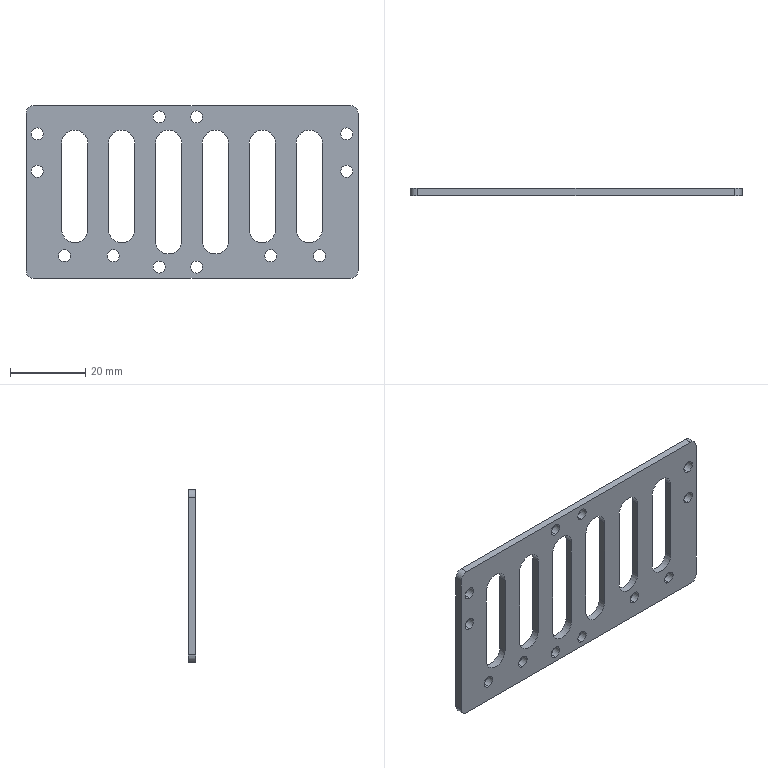Part | SolidWorks | features Extrusion 1, Fillet 1, ICE 1 | 1 solid | 64 faces | box 88.5 x 2 x 46 mm | volume 5464 mm3 | cylinder 46 | plane 18 | commonest cylinder face diameters 3.2 x24 7 x18 4 x4